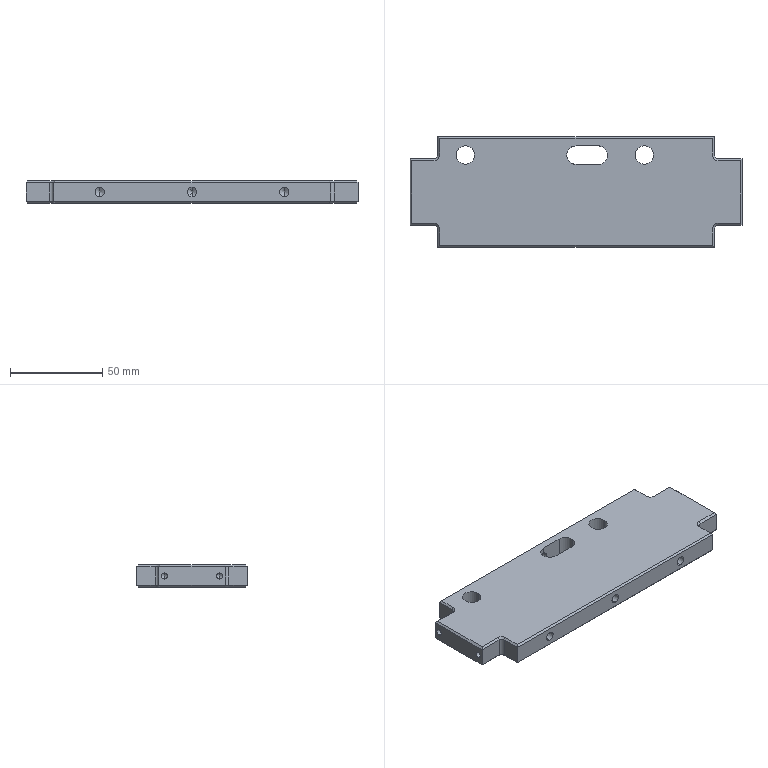Part | STEP file | 03-15 trimming support plate | 1 solid | 100 faces | box 180 x 60 x 12 mm | volume 114271 mm3 | plane 40 | cylinder 32 | cone 28 | commonest cylinder face diameters 5 x13 3.3 x8 10 x7 4 x4